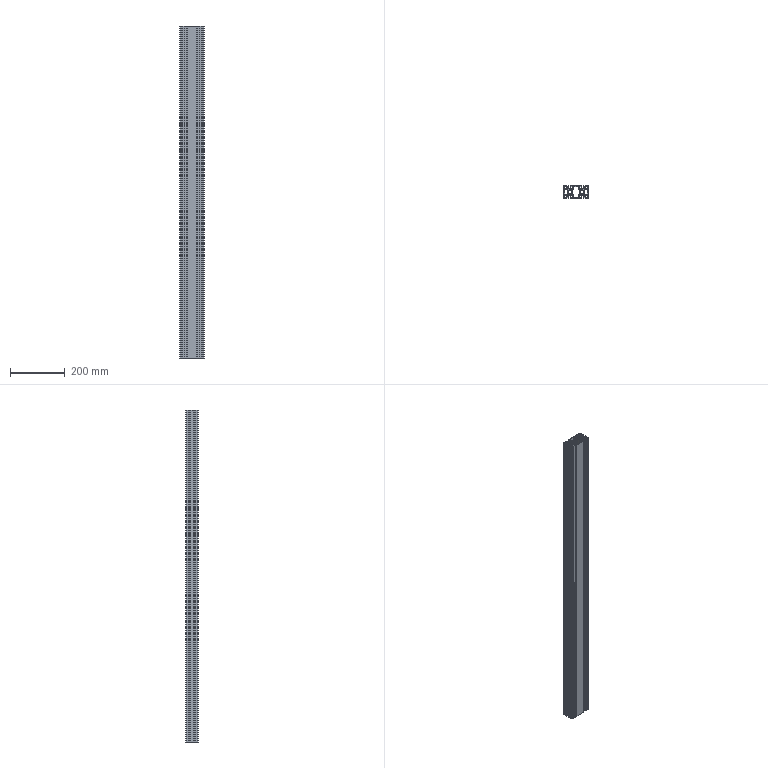Part | STEP file | 4590-1210 aluminium profile | 1 solid | 366 faces | box 90 x 45 x 1210 mm | volume 1418972 mm3 | plane 254 | cylinder 112 | commonest cylinder face diameters 2 x64 8 x20 12 x16 4 x12